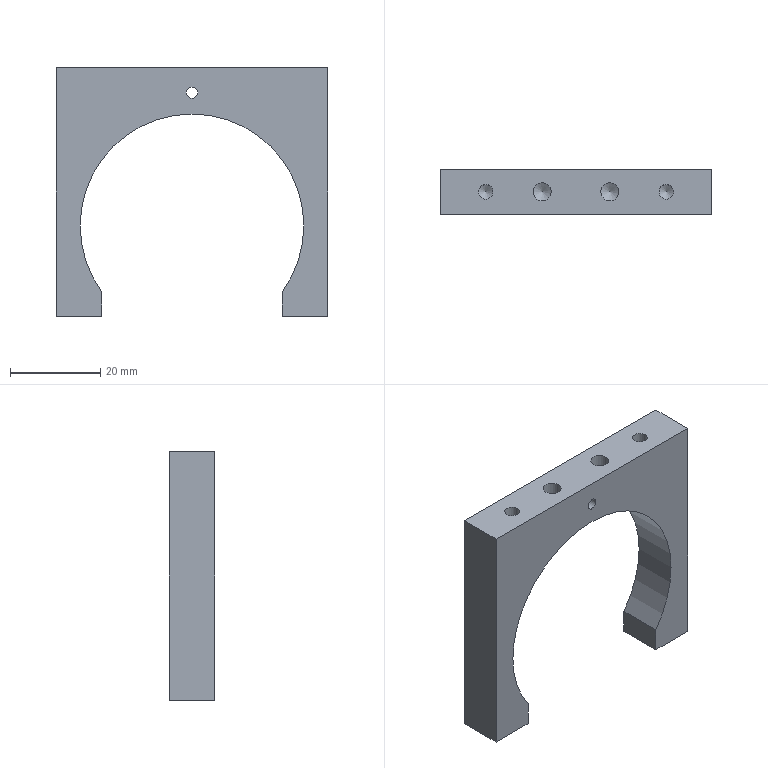Part | STEP file | SynoNew-0304-066 | 1 solid | 23 faces | box 60 x 10 x 55 mm | volume 13958 mm3 | plane 9 | cylinder 8 | cone 6 | commonest cylinder face diameters 2.46 x3 3.24 x2 4 x2 49.5 x1
STEP:
#1=CARTESIAN_POINT('',(0.,0.,-55.));
#2=VERTEX_POINT('',#1);
#3=CARTESIAN_POINT('',(0.,0.,0.));
#4=VERTEX_POINT('',#3);
#5=CARTESIAN_POINT('',(0.,0.,-55.));
#6=DIRECTION('',(0.,0.,1.));
#7=VECTOR('',#6,55.);
#8=LINE('',#5,#7);
#9=EDGE_CURVE('',#2,#4,#8,.T.);
#10=ORIENTED_EDGE('',*,*,#9,.T.);
#11=CARTESIAN_POINT('',(0.,10.,0.));
#12=VERTEX_POINT('',#11);
#13=CARTESIAN_POINT('',(0.,10.,0.));
#14=DIRECTION('',(0.,-1.,0.));
#15=VECTOR('',#14,10.);
#16=LINE('',#13,#15);
#17=EDGE_CURVE('',#12,#4,#16,.T.);
#18=ORIENTED_EDGE('',*,*,#17,.F.);
#19=CARTESIAN_POINT('',(0.,10.,-55.));
#20=VERTEX_POINT('',#19);
#21=CARTESIAN_POINT('',(0.,10.,-55.));
#22=DIRECTION('',(0.,0.,1.));
#23=VECTOR('',#22,55.);
#24=LINE('',#21,#23);
#25=EDGE_CURVE('',#20,#12,#24,.T.);
#26=ORIENTED_EDGE('',*,*,#25,.F.);
#27=CARTESIAN_POINT('',(0.,10.,-55.));
#28=DIRECTION('',(0.,-1.,0.));
#29=VECTOR('',#28,10.);
#30=LINE('',#27,#29);
#31=EDGE_CURVE('',#20,#2,#30,.T.);
#32=ORIENTED_EDGE('',*,*,#31,.T.);
#33=EDGE_LOOP('',(#10,#18,#26,#32));
#34=FACE_OUTER_BOUND('',#33,.T.);
#35=CARTESIAN_POINT('',(0.,10.,0.));
#36=DIRECTION('',(1.,0.,0.));
#37=DIRECTION('',(0.,0.,-1.));
#38=AXIS2_PLACEMENT_3D('',#35,#36,#37);
#39=PLANE('',#38);
#40=ADVANCED_FACE('',(#34),#39,.F.);
#41=CARTESIAN_POINT('',(60.,0.,0.));
#42=VERTEX_POINT('',#41);
#43=CARTESIAN_POINT('',(0.,0.,0.));
#44=DIRECTION('',(1.,0.,0.));
#45=VECTOR('',#44,60.);
#46=LINE('',#43,#45);
#47=EDGE_CURVE('',#4,#42,#46,.T.);
#48=ORIENTED_EDGE('',*,*,#47,.T.);
#49=CARTESIAN_POINT('',(60.,10.,0.));
#50=VERTEX_POINT('',#49);
#51=CARTESIAN_POINT('',(60.,10.,0.));
#52=DIRECTION('',(0.,-1.,0.));
#53=VECTOR('',#52,10.);
#54=LINE('',#51,#53);
#55=EDGE_CURVE('',#50,#42,#54,.T.);
#56=ORIENTED_EDGE('',*,*,#55,.F.);
#57=CARTESIAN_POINT('',(0.,10.,0.));
#58=DIRECTION('',(1.,0.,0.));
#59=VECTOR('',#58,60.);
#60=LINE('',#57,#59);
#61=EDGE_CURVE('',#12,#50,#60,.T.);
#62=ORIENTED_EDGE('',*,*,#61,.F.);
#63=ORIENTED_EDGE('',*,*,#17,.T.);
#64=EDGE_LOOP('',(#48,#56,#62,#63));
#65=FACE_OUTER_BOUND('',#64,.T.);
#66=CARTESIAN_POINT('',(24.5,5.,0.));
#67=VERTEX_POINT('',#66);
#68=CARTESIAN_POINT('',(20.5,5.,0.));
#69=VERTEX_POINT('',#68);
#70=CARTESIAN_POINT('',(22.5,5.,0.));
#71=DIRECTION('',(0.,0.,1.));
#72=DIRECTION('',(1.,0.,0.));
#73=AXIS2_PLACEMENT_3D('',#70,#71,#72);
#74=CIRCLE('',#73,2.);
#75=EDGE_CURVE('',#67,#69,#74,.T.);
#76=ORIENTED_EDGE('',*,*,#75,.F.);
#77=CARTESIAN_POINT('',(22.5,5.,0.));
#78=DIRECTION('',(0.,0.,1.));
#79=DIRECTION('',(1.,0.,0.));
#80=AXIS2_PLACEMENT_3D('',#77,#78,#79);
#81=CIRCLE('',#80,2.);
#82=EDGE_CURVE('',#69,#67,#81,.T.);
#83=ORIENTED_EDGE('',*,*,#82,.F.);
#84=EDGE_LOOP('',(#76,#83));
#85=FACE_BOUND('',#84,.T.);
#86=CARTESIAN_POINT('',(39.5,5.,0.));
#87=VERTEX_POINT('',#86);
#88=CARTESIAN_POINT('',(35.5,5.,0.));
#89=VERTEX_POINT('',#88);
#90=CARTESIAN_POINT('',(37.5,5.,0.));
#91=DIRECTION('',(0.,0.,1.));
#92=DIRECTION('',(1.,0.,0.));
#93=AXIS2_PLACEMENT_3D('',#90,#91,#92);
#94=CIRCLE('',#93,2.);
#95=EDGE_CURVE('',#87,#89,#94,.T.);
#96=ORIENTED_EDGE('',*,*,#95,.F.);
#97=CARTESIAN_POINT('',(37.5,5.,0.));
#98=DIRECTION('',(0.,0.,1.));
#99=DIRECTION('',(1.,0.,0.));
#100=AXIS2_PLACEMENT_3D('',#97,#98,#99);
#101=CIRCLE('',#100,2.);
#102=EDGE_CURVE('',#89,#87,#101,.T.);
#103=ORIENTED_EDGE('',*,*,#102,.F.);
#104=EDGE_LOOP('',(#96,#103));
#105=FACE_BOUND('',#104,.T.);
#106=CARTESIAN_POINT('',(51.62,5.,0.));
#107=VERTEX_POINT('',#106);
#108=CARTESIAN_POINT('',(48.38,5.,0.));
#109=VERTEX_POINT('',#108);
#110=CARTESIAN_POINT('',(50.,5.,0.));
#111=DIRECTION('',(0.,0.,1.));
#112=DIRECTION('',(1.,0.,0.));
#113=AXIS2_PLACEMENT_3D('',#110,#111,#112);
#114=CIRCLE('',#113,1.62);
#115=EDGE_CURVE('',#107,#109,#114,.T.);
#116=ORIENTED_EDGE('',*,*,#115,.F.);
#117=CARTESIAN_POINT('',(50.,5.,0.));
#118=DIRECTION('',(0.,0.,1.));
#119=DIRECTION('',(1.,0.,0.));
#120=AXIS2_PLACEMENT_3D('',#117,#118,#119);
#121=CIRCLE('',#120,1.62);
#122=EDGE_CURVE('',#109,#107,#121,.T.);
#123=ORIENTED_EDGE('',*,*,#122,.F.);
#124=EDGE_LOOP('',(#116,#123));
#125=FACE_BOUND('',#124,.T.);
#126=CARTESIAN_POINT('',(11.62,5.,0.));
#127=VERTEX_POINT('',#126);
#128=CARTESIAN_POINT('',(8.38,5.,0.));
#129=VERTEX_POINT('',#128);
#130=CARTESIAN_POINT('',(10.,5.,0.));
#131=DIRECTION('',(0.,0.,1.));
#132=DIRECTION('',(1.,0.,0.));
#133=AXIS2_PLACEMENT_3D('',#130,#131,#132);
#134=CIRCLE('',#133,1.62);
#135=EDGE_CURVE('',#127,#129,#134,.T.);
#136=ORIENTED_EDGE('',*,*,#135,.F.);
#137=CARTESIAN_POINT('',(10.,5.,0.));
#138=DIRECTION('',(0.,0.,1.));
#139=DIRECTION('',(1.,0.,0.));
#140=AXIS2_PLACEMENT_3D('',#137,#138,#139);
#141=CIRCLE('',#140,1.62);
#142=EDGE_CURVE('',#129,#127,#141,.T.);
#143=ORIENTED_EDGE('',*,*,#142,.F.);
#144=EDGE_LOOP('',(#136,#143));
#145=FACE_BOUND('',#144,.T.);
#146=CARTESIAN_POINT('',(0.,10.,0.));
#147=DIRECTION('',(0.,0.,-1.));
#148=DIRECTION('',(-1.,0.,0.));
#149=AXIS2_PLACEMENT_3D('',#146,#147,#148);
#150=PLANE('',#149);
#151=ADVANCED_FACE('',(#65,#85,#105,#125,#145),#150,.F.);
#152=CARTESIAN_POINT('',(60.,0.,-55.));
#153=VERTEX_POINT('',#152);
#154=CARTESIAN_POINT('',(60.,0.,0.));
#155=DIRECTION('',(0.,0.,-1.));
#156=VECTOR('',#155,55.);
#157=LINE('',#154,#156);
#158=EDGE_CURVE('',#42,#153,#157,.T.);
#159=ORIENTED_EDGE('',*,*,#158,.T.);
#160=CARTESIAN_POINT('',(60.,10.,-55.));
#161=VERTEX_POINT('',#160);
#162=CARTESIAN_POINT('',(60.,10.,-55.));
#163=DIRECTION('',(0.,-1.,0.));
#164=VECTOR('',#163,10.);
#165=LINE('',#162,#164);
#166=EDGE_CURVE('',#161,#153,#165,.T.);
#167=ORIENTED_EDGE('',*,*,#166,.F.);
#168=CARTESIAN_POINT('',(60.,10.,0.));
#169=DIRECTION('',(0.,0.,-1.));
#170=VECTOR('',#169,55.);
#171=LINE('',#168,#170);
#172=EDGE_CURVE('',#50,#161,#171,.T.);
#173=ORIENTED_EDGE('',*,*,#172,.F.);
#174=ORIENTED_EDGE('',*,*,#55,.T.);
#175=EDGE_LOOP('',(#159,#167,#173,#174));
#176=FACE_OUTER_BOUND('',#175,.T.);
#177=CARTESIAN_POINT('',(60.,10.,0.));
#178=DIRECTION('',(-1.,0.,0.));
#179=DIRECTION('',(0.,0.,1.));
#180=AXIS2_PLACEMENT_3D('',#177,#178,#179);
#181=PLANE('',#180);
#182=ADVANCED_FACE('',(#176),#181,.F.);
#183=CARTESIAN_POINT('',(50.,0.,-55.));
#184=VERTEX_POINT('',#183);
#185=CARTESIAN_POINT('',(60.,0.,-55.));
#186=DIRECTION('',(-1.,0.,0.));
#187=VECTOR('',#186,10.);
#188=LINE('',#185,#187);
#189=EDGE_CURVE('',#153,#184,#188,.T.);
#190=ORIENTED_EDGE('',*,*,#189,.T.);
#191=CARTESIAN_POINT('',(50.,10.,-55.));
#192=VERTEX_POINT('',#191);
#193=CARTESIAN_POINT('',(50.,10.,-55.));
#194=DIRECTION('',(0.,-1.,0.));
#195=VECTOR('',#194,10.);
#196=LINE('',#193,#195);
#197=EDGE_CURVE('',#192,#184,#196,.T.);
#198=ORIENTED_EDGE('',*,*,#197,.F.);
#199=CARTESIAN_POINT('',(60.,10.,-55.));
#200=DIRECTION('',(-1.,0.,0.));
#201=VECTOR('',#200,10.);
#202=LINE('',#199,#201);
#203=EDGE_CURVE('',#161,#192,#202,.T.);
#204=ORIENTED_EDGE('',*,*,#203,.F.);
#205=ORIENTED_EDGE('',*,*,#166,.T.);
#206=EDGE_LOOP('',(#190,#198,#204,#205));
#207=FACE_OUTER_BOUND('',#206,.T.);
#208=CARTESIAN_POINT('',(53.77,5.,-55.));
#209=VERTEX_POINT('',#208);
#210=CARTESIAN_POINT('',(56.23,5.,-55.));
#211=VERTEX_POINT('',#210);
#212=CARTESIAN_POINT('',(55.,5.,-55.));
#213=DIRECTION('',(0.,0.,-1.));
#214=DIRECTION('',(-1.,0.,0.));
#215=AXIS2_PLACEMENT_3D('',#212,#213,#214);
#216=CIRCLE('',#215,1.23);
#217=EDGE_CURVE('',#209,#211,#216,.T.);
#218=ORIENTED_EDGE('',*,*,#217,.F.);
#219=CARTESIAN_POINT('',(55.,5.,-55.));
#220=DIRECTION('',(0.,0.,-1.));
#221=DIRECTION('',(-1.,0.,0.));
#222=AXIS2_PLACEMENT_3D('',#219,#220,#221);
#223=CIRCLE('',#222,1.23);
#224=EDGE_CURVE('',#211,#209,#223,.T.);
#225=ORIENTED_EDGE('',*,*,#224,.F.);
#226=EDGE_LOOP('',(#218,#225));
#227=FACE_BOUND('',#226,.T.);
#228=CARTESIAN_POINT('',(50.,10.,-55.));
#229=DIRECTION('',(0.,0.,1.));
#230=DIRECTION('',(1.,0.,0.));
#231=AXIS2_PLACEMENT_3D('',#228,#229,#230);
#232=PLANE('',#231);
#233=ADVANCED_FACE('',(#207,#227),#232,.F.);
#234=CARTESIAN_POINT('',(50.,0.,-49.58));
#235=VERTEX_POINT('',#234);
#236=CARTESIAN_POINT('',(50.,0.,-55.));
#237=DIRECTION('',(0.,0.,1.));
#238=VECTOR('',#237,5.42);
#239=LINE('',#236,#238);
#240=EDGE_CURVE('',#184,#235,#239,.T.);
#241=ORIENTED_EDGE('',*,*,#240,.T.);
#242=CARTESIAN_POINT('',(50.,10.,-49.58));
#243=VERTEX_POINT('',#242);
#244=CARTESIAN_POINT('',(50.,10.,-49.58));
#245=DIRECTION('',(0.,-1.,0.));
#246=VECTOR('',#245,10.);
#247=LINE('',#244,#246);
#248=EDGE_CURVE('',#243,#235,#247,.T.);
#249=ORIENTED_EDGE('',*,*,#248,.F.);
#250=CARTESIAN_POINT('',(50.,10.,-55.));
#251=DIRECTION('',(0.,0.,1.));
#252=VECTOR('',#251,5.42);
#253=LINE('',#250,#252);
#254=EDGE_CURVE('',#192,#243,#253,.T.);
#255=ORIENTED_EDGE('',*,*,#254,.F.);
#256=ORIENTED_EDGE('',*,*,#197,.T.);
#257=EDGE_LOOP('',(#241,#249,#255,#256));
#258=FACE_OUTER_BOUND('',#257,.T.);
#259=CARTESIAN_POINT('',(50.,10.,-55.));
#260=DIRECTION('',(1.,0.,0.));
#261=DIRECTION('',(0.,0.,-1.));
#262=AXIS2_PLACEMENT_3D('',#259,#260,#261);
#263=PLANE('',#262);
#264=ADVANCED_FACE('',(#258),#263,.F.);
#265=CARTESIAN_POINT('',(10.,0.,-49.58));
#266=VERTEX_POINT('',#265);
#267=CARTESIAN_POINT('',(30.,0.,-35.));
#268=DIRECTION('',(0.,-1.,0.));
#269=DIRECTION('',(0.,0.,1.));
#270=AXIS2_PLACEMENT_3D('',#267,#268,#269);
#271=CIRCLE('',#270,24.75);
#272=EDGE_CURVE('',#235,#266,#271,.T.);
#273=ORIENTED_EDGE('',*,*,#272,.T.);
#274=CARTESIAN_POINT('',(10.,10.,-49.58));
#275=VERTEX_POINT('',#274);
#276=CARTESIAN_POINT('',(10.,10.,-49.58));
#277=DIRECTION('',(0.,-1.,0.));
#278=VECTOR('',#277,10.);
#279=LINE('',#276,#278);
#280=EDGE_CURVE('',#275,#266,#279,.T.);
#281=ORIENTED_EDGE('',*,*,#280,.F.);
#282=CARTESIAN_POINT('',(30.,10.,-35.));
#283=DIRECTION('',(0.,-1.,0.));
#284=DIRECTION('',(0.,0.,1.));
#285=AXIS2_PLACEMENT_3D('',#282,#283,#284);
#286=CIRCLE('',#285,24.75);
#287=EDGE_CURVE('',#243,#275,#286,.T.);
#288=ORIENTED_EDGE('',*,*,#287,.F.);
#289=ORIENTED_EDGE('',*,*,#248,.T.);
#290=EDGE_LOOP('',(#273,#281,#288,#289));
#291=FACE_OUTER_BOUND('',#290,.T.);
#292=CARTESIAN_POINT('',(30.,10.,-35.));
#293=DIRECTION('',(0.,-1.,0.));
#294=DIRECTION('',(0.,0.,1.));
#295=AXIS2_PLACEMENT_3D('',#292,#293,#294);
#296=CYLINDRICAL_SURFACE('',#295,24.75);
#297=ADVANCED_FACE('',(#291),#296,.F.);
#298=CARTESIAN_POINT('',(10.,0.,-55.));
#299=VERTEX_POINT('',#298);
#300=CARTESIAN_POINT('',(10.,0.,-49.58));
#301=DIRECTION('',(0.,0.,-1.));
#302=VECTOR('',#301,5.42);
#303=LINE('',#300,#302);
#304=EDGE_CURVE('',#266,#299,#303,.T.);
#305=ORIENTED_EDGE('',*,*,#304,.T.);
#306=CARTESIAN_POINT('',(10.,10.,-55.));
#307=VERTEX_POINT('',#306);
#308=CARTESIAN_POINT('',(10.,10.,-55.));
#309=DIRECTION('',(0.,-1.,0.));
#310=VECTOR('',#309,10.);
#311=LINE('',#308,#310);
#312=EDGE_CURVE('',#307,#299,#311,.T.);
#313=ORIENTED_EDGE('',*,*,#312,.F.);
#314=CARTESIAN_POINT('',(10.,10.,-49.58));
#315=DIRECTION('',(0.,0.,-1.));
#316=VECTOR('',#315,5.42);
#317=LINE('',#314,#316);
#318=EDGE_CURVE('',#275,#307,#317,.T.);
#319=ORIENTED_EDGE('',*,*,#318,.F.);
#320=ORIENTED_EDGE('',*,*,#280,.T.);
#321=EDGE_LOOP('',(#305,#313,#319,#320));
#322=FACE_OUTER_BOUND('',#321,.T.);
#323=CARTESIAN_POINT('',(10.,10.,-55.));
#324=DIRECTION('',(-1.,0.,0.));
#325=DIRECTION('',(0.,0.,1.));
#326=AXIS2_PLACEMENT_3D('',#323,#324,#325);
#327=PLANE('',#326);
#328=ADVANCED_FACE('',(#322),#327,.F.);
#329=CARTESIAN_POINT('',(10.,0.,-55.));
#330=DIRECTION('',(-1.,0.,0.));
#331=VECTOR('',#330,10.);
#332=LINE('',#329,#331);
#333=EDGE_CURVE('',#299,#2,#332,.T.);
#334=ORIENTED_EDGE('',*,*,#333,.T.);
#335=ORIENTED_EDGE('',*,*,#31,.F.);
#336=CARTESIAN_POINT('',(10.,10.,-55.));
#337=DIRECTION('',(-1.,0.,0.));
#338=VECTOR('',#337,10.);
#339=LINE('',#336,#338);
#340=EDGE_CURVE('',#307,#20,#339,.T.);
#341=ORIENTED_EDGE('',*,*,#340,.F.);
#342=ORIENTED_EDGE('',*,*,#312,.T.);
#343=EDGE_LOOP('',(#334,#335,#341,#342));
#344=FACE_OUTER_BOUND('',#343,.T.);
#345=CARTESIAN_POINT('',(3.77,5.,-55.));
#346=VERTEX_POINT('',#345);
#347=CARTESIAN_POINT('',(6.23,5.,-55.));
#348=VERTEX_POINT('',#347);
#349=CARTESIAN_POINT('',(5.,5.,-55.));
#350=DIRECTION('',(0.,0.,-1.));
#351=DIRECTION('',(-1.,0.,0.));
#352=AXIS2_PLACEMENT_3D('',#349,#350,#351);
#353=CIRCLE('',#352,1.23);
#354=EDGE_CURVE('',#346,#348,#353,.T.);
#355=ORIENTED_EDGE('',*,*,#354,.F.);
#356=CARTESIAN_POINT('',(5.,5.,-55.));
#357=DIRECTION('',(0.,0.,-1.));
#358=DIRECTION('',(-1.,0.,0.));
#359=AXIS2_PLACEMENT_3D('',#356,#357,#358);
#360=CIRCLE('',#359,1.23);
#361=EDGE_CURVE('',#348,#346,#360,.T.);
#362=ORIENTED_EDGE('',*,*,#361,.F.);
#363=EDGE_LOOP('',(#355,#362));
#364=FACE_BOUND('',#363,.T.);
#365=CARTESIAN_POINT('',(0.,10.,-55.));
#366=DIRECTION('',(0.,0.,1.));
#367=DIRECTION('',(1.,0.,0.));
#368=AXIS2_PLACEMENT_3D('',#365,#366,#367);
#369=PLANE('',#368);
#370=ADVANCED_FACE('',(#344,#364),#369,.F.);
#371=ORIENTED_EDGE('',*,*,#25,.T.);
#372=ORIENTED_EDGE('',*,*,#61,.T.);
#373=ORIENTED_EDGE('',*,*,#172,.T.);
#374=ORIENTED_EDGE('',*,*,#203,.T.);
#375=ORIENTED_EDGE('',*,*,#254,.T.);
#376=ORIENTED_EDGE('',*,*,#287,.T.);
#377=ORIENTED_EDGE('',*,*,#318,.T.);
#378=ORIENTED_EDGE('',*,*,#340,.T.);
#379=EDGE_LOOP('',(#371,#372,#373,#374,#375,#376,#377,#378));
#380=FACE_OUTER_BOUND('',#379,.T.);
#381=CARTESIAN_POINT('',(30.,10.,-4.27));
#382=VERTEX_POINT('',#381);
#383=CARTESIAN_POINT('',(30.,10.,-6.73));
#384=VERTEX_POINT('',#383);
#385=CARTESIAN_POINT('',(30.,10.,-5.5));
#386=DIRECTION('',(0.,1.,0.));
#387=DIRECTION('',(0.,0.,1.));
#388=AXIS2_PLACEMENT_3D('',#385,#386,#387);
#389=CIRCLE('',#388,1.23);
#390=EDGE_CURVE('',#382,#384,#389,.T.);
#391=ORIENTED_EDGE('',*,*,#390,.F.);
#392=CARTESIAN_POINT('',(30.,10.,-5.5));
#393=DIRECTION('',(0.,1.,0.));
#394=DIRECTION('',(0.,0.,1.));
#395=AXIS2_PLACEMENT_3D('',#392,#393,#394);
#396=CIRCLE('',#395,1.23);
#397=EDGE_CURVE('',#384,#382,#396,.T.);
#398=ORIENTED_EDGE('',*,*,#397,.F.);
#399=EDGE_LOOP('',(#391,#398));
#400=FACE_BOUND('',#399,.T.);
#401=CARTESIAN_POINT('',(30.,10.,-35.));
#402=DIRECTION('',(0.,1.,0.));
#403=DIRECTION('',(0.,0.,1.));
#404=AXIS2_PLACEMENT_3D('',#401,#402,#403);
#405=PLANE('',#404);
#406=ADVANCED_FACE('',(#380,#400),#405,.T.);
#407=ORIENTED_EDGE('',*,*,#9,.F.);
#408=ORIENTED_EDGE('',*,*,#333,.F.);
#409=ORIENTED_EDGE('',*,*,#304,.F.);
#410=ORIENTED_EDGE('',*,*,#272,.F.);
#411=ORIENTED_EDGE('',*,*,#240,.F.);
#412=ORIENTED_EDGE('',*,*,#189,.F.);
#413=ORIENTED_EDGE('',*,*,#158,.F.);
#414=ORIENTED_EDGE('',*,*,#47,.F.);
#415=EDGE_LOOP('',(#407,#408,#409,#410,#411,#412,#413,#414));
#416=FACE_OUTER_BOUND('',#415,.T.);
#417=CARTESIAN_POINT('',(30.,0.,-4.27));
#418=VERTEX_POINT('',#417);
#419=CARTESIAN_POINT('',(30.,0.,-6.73));
#420=VERTEX_POINT('',#419);
#421=CARTESIAN_POINT('',(30.,0.,-5.5));
#422=DIRECTION('',(0.,1.,0.));
#423=DIRECTION('',(0.,0.,1.));
#424=AXIS2_PLACEMENT_3D('',#421,#422,#423);
#425=CIRCLE('',#424,1.23);
#426=EDGE_CURVE('',#418,#420,#425,.T.);
#427=ORIENTED_EDGE('',*,*,#426,.T.);
#428=CARTESIAN_POINT('',(30.,0.,-5.5));
#429=DIRECTION('',(0.,1.,0.));
#430=DIRECTION('',(0.,0.,1.));
#431=AXIS2_PLACEMENT_3D('',#428,#429,#430);
#432=CIRCLE('',#431,1.23);
#433=EDGE_CURVE('',#420,#418,#432,.T.);
#434=ORIENTED_EDGE('',*,*,#433,.T.);
#435=EDGE_LOOP('',(#427,#434));
#436=FACE_BOUND('',#435,.T.);
#437=CARTESIAN_POINT('',(30.,0.,-35.));
#438=DIRECTION('',(0.,1.,0.));
#439=DIRECTION('',(0.,0.,1.));
#440=AXIS2_PLACEMENT_3D('',#437,#438,#439);
#441=PLANE('',#440);
#442=ADVANCED_FACE('',(#416,#436),#441,.F.);
#443=CARTESIAN_POINT('',(10.,5.,-12.473));
#444=VERTEX_POINT('',#443);
#445=CARTESIAN_POINT('',(8.38,5.,-11.5));
#446=VERTEX_POINT('',#445);
#447=CARTESIAN_POINT('',(8.38,5.,-11.5));
#448=DIRECTION('',(-0.8572,0.,0.515));
#449=VECTOR('',#448,1.62);
#450=LINE('',#447,#449);
#451=EDGE_CURVE('',#444,#446,#450,.T.);
#452=ORIENTED_EDGE('',*,*,#451,.T.);
#453=CARTESIAN_POINT('',(11.62,5.,-11.5));
#454=VERTEX_POINT('',#453);
#455=CARTESIAN_POINT('',(10.,5.,-11.5));
#456=DIRECTION('',(0.,0.,1.));
#457=DIRECTION('',(1.,0.,0.));
#458=AXIS2_PLACEMENT_3D('',#455,#456,#457);
#459=CIRCLE('',#458,1.62);
#460=EDGE_CURVE('',#446,#454,#459,.T.);
#461=ORIENTED_EDGE('',*,*,#460,.T.);
#462=CARTESIAN_POINT('',(10.,5.,-11.5));
#463=DIRECTION('',(0.,0.,1.));
#464=DIRECTION('',(1.,0.,0.));
#465=AXIS2_PLACEMENT_3D('',#462,#463,#464);
#466=CIRCLE('',#465,1.62);
#467=EDGE_CURVE('',#454,#446,#466,.T.);
#468=ORIENTED_EDGE('',*,*,#467,.T.);
#469=ORIENTED_EDGE('',*,*,#451,.F.);
#470=EDGE_LOOP('',(#452,#461,#468,#469));
#471=FACE_OUTER_BOUND('',#470,.T.);
#472=CARTESIAN_POINT('',(10.,5.,-11.5));
#473=DIRECTION('',(0.,0.,1.));
#474=DIRECTION('',(1.,0.,0.));
#475=AXIS2_PLACEMENT_3D('',#472,#473,#474);
#476=CONICAL_SURFACE('',#475,1.62,1.03);
#477=ADVANCED_FACE('',(#471),#476,.F.);
#478=ORIENTED_EDGE('',*,*,#467,.F.);
#479=ORIENTED_EDGE('',*,*,#460,.F.);
#480=CARTESIAN_POINT('',(8.38,5.,0.));
#481=DIRECTION('',(0.,0.,1.));
#482=VECTOR('',#481,1.62);
#483=LINE('',#480,#482);
#484=EDGE_CURVE('',#446,#129,#483,.T.);
#485=ORIENTED_EDGE('',*,*,#484,.T.);
#486=ORIENTED_EDGE('',*,*,#142,.T.);
#487=ORIENTED_EDGE('',*,*,#135,.T.);
#488=ORIENTED_EDGE('',*,*,#484,.F.);
#489=EDGE_LOOP('',(#478,#479,#485,#486,#487,#488));
#490=FACE_OUTER_BOUND('',#489,.T.);
#491=CARTESIAN_POINT('',(10.,5.,0.));
#492=DIRECTION('',(0.,0.,1.));
#493=DIRECTION('',(1.,0.,0.));
#494=AXIS2_PLACEMENT_3D('',#491,#492,#493);
#495=CYLINDRICAL_SURFACE('',#494,1.62);
#496=ADVANCED_FACE('',(#490),#495,.F.);
#497=CARTESIAN_POINT('',(50.,5.,-12.473));
#498=VERTEX_POINT('',#497);
#499=CARTESIAN_POINT('',(48.38,5.,-11.5));
#500=VERTEX_POINT('',#499);
#501=CARTESIAN_POINT('',(48.38,5.,-11.5));
#502=DIRECTION('',(-0.8572,0.,0.515));
#503=VECTOR('',#502,1.62);
#504=LINE('',#501,#503);
#505=EDGE_CURVE('',#498,#500,#504,.T.);
#506=ORIENTED_EDGE('',*,*,#505,.T.);
#507=CARTESIAN_POINT('',(51.62,5.,-11.5));
#508=VERTEX_POINT('',#507);
#509=CARTESIAN_POINT('',(50.,5.,-11.5));
#510=DIRECTION('',(0.,0.,1.));
#511=DIRECTION('',(1.,0.,0.));
#512=AXIS2_PLACEMENT_3D('',#509,#510,#511);
#513=CIRCLE('',#512,1.62);
#514=EDGE_CURVE('',#500,#508,#513,.T.);
#515=ORIENTED_EDGE('',*,*,#514,.T.);
#516=CARTESIAN_POINT('',(50.,5.,-11.5));
#517=DIRECTION('',(0.,0.,1.));
#518=DIRECTION('',(1.,0.,0.));
#519=AXIS2_PLACEMENT_3D('',#516,#517,#518);
#520=CIRCLE('',#519,1.62);
#521=EDGE_CURVE('',#508,#500,#520,.T.);
#522=ORIENTED_EDGE('',*,*,#521,.T.);
#523=ORIENTED_EDGE('',*,*,#505,.F.);
#524=EDGE_LOOP('',(#506,#515,#522,#523));
#525=FACE_OUTER_BOUND('',#524,.T.);
#526=CARTESIAN_POINT('',(50.,5.,-11.5));
#527=DIRECTION('',(0.,0.,1.));
#528=DIRECTION('',(1.,0.,0.));
#529=AXIS2_PLACEMENT_3D('',#526,#527,#528);
#530=CONICAL_SURFACE('',#529,1.62,1.03);
#531=ADVANCED_FACE('',(#525),#530,.F.);
#532=ORIENTED_EDGE('',*,*,#521,.F.);
#533=ORIENTED_EDGE('',*,*,#514,.F.);
#534=CARTESIAN_POINT('',(48.38,5.,0.));
#535=DIRECTION('',(0.,0.,1.));
#536=VECTOR('',#535,1.62);
#537=LINE('',#534,#536);
#538=EDGE_CURVE('',#500,#109,#537,.T.);
#539=ORIENTED_EDGE('',*,*,#538,.T.);
#540=ORIENTED_EDGE('',*,*,#122,.T.);
#541=ORIENTED_EDGE('',*,*,#115,.T.);
#542=ORIENTED_EDGE('',*,*,#538,.F.);
#543=EDGE_LOOP('',(#532,#533,#539,#540,#541,#542));
#544=FACE_OUTER_BOUND('',#543,.T.);
#545=CARTESIAN_POINT('',(50.,5.,0.));
#546=DIRECTION('',(0.,0.,1.));
#547=DIRECTION('',(1.,0.,0.));
#548=AXIS2_PLACEMENT_3D('',#545,#546,#547);
#549=CYLINDRICAL_SURFACE('',#548,1.62);
#550=ADVANCED_FACE('',(#544),#549,.F.);
#551=CARTESIAN_POINT('',(37.5,5.,-7.202));
#552=VERTEX_POINT('',#551);
#553=CARTESIAN_POINT('',(35.5,5.,-6.));
#554=VERTEX_POINT('',#553);
#555=CARTESIAN_POINT('',(35.5,5.,-6.));
#556=DIRECTION('',(-0.8572,0.,0.515));
#557=VECTOR('',#556,2.);
#558=LINE('',#555,#557);
#559=EDGE_CURVE('',#552,#554,#558,.T.);
#560=ORIENTED_EDGE('',*,*,#559,.T.);
#561=CARTESIAN_POINT('',(39.5,5.,-6.));
#562=VERTEX_POINT('',#561);
#563=CARTESIAN_POINT('',(37.5,5.,-6.));
#564=DIRECTION('',(0.,0.,1.));
#565=DIRECTION('',(1.,0.,0.));
#566=AXIS2_PLACEMENT_3D('',#563,#564,#565);
#567=CIRCLE('',#566,2.);
#568=EDGE_CURVE('',#554,#562,#567,.T.);
#569=ORIENTED_EDGE('',*,*,#568,.T.);
#570=CARTESIAN_POINT('',(37.5,5.,-6.));
#571=DIRECTION('',(0.,0.,1.));
#572=DIRECTION('',(1.,0.,0.));
#573=AXIS2_PLACEMENT_3D('',#570,#571,#572);
#574=CIRCLE('',#573,2.);
#575=EDGE_CURVE('',#562,#554,#574,.T.);
#576=ORIENTED_EDGE('',*,*,#575,.T.);
#577=ORIENTED_EDGE('',*,*,#559,.F.);
#578=EDGE_LOOP('',(#560,#569,#576,#577));
#579=FACE_OUTER_BOUND('',#578,.T.);
#580=CARTESIAN_POINT('',(37.5,5.,-6.));
#581=DIRECTION('',(0.,0.,1.));
#582=DIRECTION('',(1.,0.,0.));
#583=AXIS2_PLACEMENT_3D('',#580,#581,#582);
#584=CONICAL_SURFACE('',#583,2.,1.03);
#585=ADVANCED_FACE('',(#579),#584,.F.);
#586=ORIENTED_EDGE('',*,*,#575,.F.);
#587=ORIENTED_EDGE('',*,*,#568,.F.);
#588=CARTESIAN_POINT('',(35.5,5.,0.));
#589=DIRECTION('',(0.,0.,1.));
#590=VECTOR('',#589,2.);
#591=LINE('',#588,#590);
#592=EDGE_CURVE('',#554,#89,#591,.T.);
#593=ORIENTED_EDGE('',*,*,#592,.T.);
#594=ORIENTED_EDGE('',*,*,#102,.T.);
#595=ORIENTED_EDGE('',*,*,#95,.T.);
#596=ORIENTED_EDGE('',*,*,#592,.F.);
#597=EDGE_LOOP('',(#586,#587,#593,#594,#595,#596));
#598=FACE_OUTER_BOUND('',#597,.T.);
#599=CARTESIAN_POINT('',(37.5,5.,0.));
#600=DIRECTION('',(0.,0.,1.));
#601=DIRECTION('',(1.,0.,0.));
#602=AXIS2_PLACEMENT_3D('',#599,#600,#601);
#603=CYLINDRICAL_SURFACE('',#602,2.);
#604=ADVANCED_FACE('',(#598),#603,.F.);
#605=CARTESIAN_POINT('',(22.5,5.,-7.202));
#606=VERTEX_POINT('',#605);
#607=CARTESIAN_POINT('',(20.5,5.,-6.));
#608=VERTEX_POINT('',#607);
#609=CARTESIAN_POINT('',(20.5,5.,-6.));
#610=DIRECTION('',(-0.8572,0.,0.515));
#611=VECTOR('',#610,2.);
#612=LINE('',#609,#611);
#613=EDGE_CURVE('',#606,#608,#612,.T.);
#614=ORIENTED_EDGE('',*,*,#613,.T.);
#615=CARTESIAN_POINT('',(24.5,5.,-6.));
#616=VERTEX_POINT('',#615);
#617=CARTESIAN_POINT('',(22.5,5.,-6.));
#618=DIRECTION('',(0.,0.,1.));
#619=DIRECTION('',(1.,0.,0.));
#620=AXIS2_PLACEMENT_3D('',#617,#618,#619);
#621=CIRCLE('',#620,2.);
#622=EDGE_CURVE('',#608,#616,#621,.T.);
#623=ORIENTED_EDGE('',*,*,#622,.T.);
#624=CARTESIAN_POINT('',(22.5,5.,-6.));
#625=DIRECTION('',(0.,0.,1.));
#626=DIRECTION('',(1.,0.,0.));
#627=AXIS2_PLACEMENT_3D('',#624,#625,#626);
#628=CIRCLE('',#627,2.);
#629=EDGE_CURVE('',#616,#608,#628,.T.);
#630=ORIENTED_EDGE('',*,*,#629,.T.);
#631=ORIENTED_EDGE('',*,*,#613,.F.);
#632=EDGE_LOOP('',(#614,#623,#630,#631));
#633=FACE_OUTER_BOUND('',#632,.T.);
#634=CARTESIAN_POINT('',(22.5,5.,-6.));
#635=DIRECTION('',(0.,0.,1.));
#636=DIRECTION('',(1.,0.,0.));
#637=AXIS2_PLACEMENT_3D('',#634,#635,#636);
#638=CONICAL_SURFACE('',#637,2.,1.03);
#639=ADVANCED_FACE('',(#633),#638,.F.);
#640=ORIENTED_EDGE('',*,*,#629,.F.);
#641=ORIENTED_EDGE('',*,*,#622,.F.);
#642=CARTESIAN_POINT('',(20.5,5.,0.));
#643=DIRECTION('',(0.,0.,1.));
#644=VECTOR('',#643,2.);
#645=LINE('',#642,#644);
#646=EDGE_CURVE('',#608,#69,#645,.T.);
#647=ORIENTED_EDGE('',*,*,#646,.T.);
#648=ORIENTED_EDGE('',*,*,#82,.T.);
#649=ORIENTED_EDGE('',*,*,#75,.T.);
#650=ORIENTED_EDGE('',*,*,#646,.F.);
#651=EDGE_LOOP('',(#640,#641,#647,#648,#649,#650));
#652=FACE_OUTER_BOUND('',#651,.T.);
#653=CARTESIAN_POINT('',(22.5,5.,0.));
#654=DIRECTION('',(0.,0.,1.));
#655=DIRECTION('',(1.,0.,0.));
#656=AXIS2_PLACEMENT_3D('',#653,#654,#655);
#657=CYLINDRICAL_SURFACE('',#656,2.);
#658=ADVANCED_FACE('',(#652),#657,.F.);
#659=CARTESIAN_POINT('',(55.,5.,-46.761));
#660=VERTEX_POINT('',#659);
#661=CARTESIAN_POINT('',(56.23,5.,-47.5));
#662=VERTEX_POINT('',#661);
#663=CARTESIAN_POINT('',(56.23,5.,-47.5));
#664=DIRECTION('',(0.8572,0.,-0.515));
#665=VECTOR('',#664,1.23);
#666=LINE('',#663,#665);
#667=EDGE_CURVE('',#660,#662,#666,.T.);
#668=ORIENTED_EDGE('',*,*,#667,.T.);
#669=CARTESIAN_POINT('',(53.77,5.,-47.5));
#670=VERTEX_POINT('',#669);
#671=CARTESIAN_POINT('',(55.,5.,-47.5));
#672=DIRECTION('',(0.,0.,-1.));
#673=DIRECTION('',(-1.,0.,0.));
#674=AXIS2_PLACEMENT_3D('',#671,#672,#673);
#675=CIRCLE('',#674,1.23);
#676=EDGE_CURVE('',#662,#670,#675,.T.);
#677=ORIENTED_EDGE('',*,*,#676,.T.);
#678=CARTESIAN_POINT('',(55.,5.,-47.5));
#679=DIRECTION('',(0.,0.,-1.));
#680=DIRECTION('',(-1.,0.,0.));
#681=AXIS2_PLACEMENT_3D('',#678,#679,#680);
#682=CIRCLE('',#681,1.23);
#683=EDGE_CURVE('',#670,#662,#682,.T.);
#684=ORIENTED_EDGE('',*,*,#683,.T.);
#685=ORIENTED_EDGE('',*,*,#667,.F.);
#686=EDGE_LOOP('',(#668,#677,#684,#685));
#687=FACE_OUTER_BOUND('',#686,.T.);
#688=CARTESIAN_POINT('',(55.,5.,-47.5));
#689=DIRECTION('',(0.,0.,-1.));
#690=DIRECTION('',(-1.,0.,0.));
#691=AXIS2_PLACEMENT_3D('',#688,#689,#690);
#692=CONICAL_SURFACE('',#691,1.23,1.03);
#693=ADVANCED_FACE('',(#687),#692,.F.);
#694=ORIENTED_EDGE('',*,*,#683,.F.);
#695=ORIENTED_EDGE('',*,*,#676,.F.);
#696=CARTESIAN_POINT('',(56.23,5.,-55.));
#697=DIRECTION('',(0.,0.,-1.));
#698=VECTOR('',#697,1.23);
#699=LINE('',#696,#698);
#700=EDGE_CURVE('',#662,#211,#699,.T.);
#701=ORIENTED_EDGE('',*,*,#700,.T.);
#702=ORIENTED_EDGE('',*,*,#224,.T.);
#703=ORIENTED_EDGE('',*,*,#217,.T.);
#704=ORIENTED_EDGE('',*,*,#700,.F.);
#705=EDGE_LOOP('',(#694,#695,#701,#702,#703,#704));
#706=FACE_OUTER_BOUND('',#705,.T.);
#707=CARTESIAN_POINT('',(55.,5.,-55.));
#708=DIRECTION('',(0.,0.,-1.));
#709=DIRECTION('',(-1.,0.,0.));
#710=AXIS2_PLACEMENT_3D('',#707,#708,#709);
#711=CYLINDRICAL_SURFACE('',#710,1.23);
#712=ADVANCED_FACE('',(#706),#711,.F.);
#713=CARTESIAN_POINT('',(5.,5.,-46.761));
#714=VERTEX_POINT('',#713);
#715=CARTESIAN_POINT('',(6.23,5.,-47.5));
#716=VERTEX_POINT('',#715);
#717=CARTESIAN_POINT('',(6.23,5.,-47.5));
#718=DIRECTION('',(0.8572,0.,-0.515));
#719=VECTOR('',#718,1.23);
#720=LINE('',#717,#719);
#721=EDGE_CURVE('',#714,#716,#720,.T.);
#722=ORIENTED_EDGE('',*,*,#721,.T.);
#723=CARTESIAN_POINT('',(3.77,5.,-47.5));
#724=VERTEX_POINT('',#723);
#725=CARTESIAN_POINT('',(5.,5.,-47.5));
#726=DIRECTION('',(0.,0.,-1.));
#727=DIRECTION('',(-1.,0.,0.));
#728=AXIS2_PLACEMENT_3D('',#725,#726,#727);
#729=CIRCLE('',#728,1.23);
#730=EDGE_CURVE('',#716,#724,#729,.T.);
#731=ORIENTED_EDGE('',*,*,#730,.T.);
#732=CARTESIAN_POINT('',(5.,5.,-47.5));
#733=DIRECTION('',(0.,0.,-1.));
#734=DIRECTION('',(-1.,0.,0.));
#735=AXIS2_PLACEMENT_3D('',#732,#733,#734);
#736=CIRCLE('',#735,1.23);
#737=EDGE_CURVE('',#724,#716,#736,.T.);
#738=ORIENTED_EDGE('',*,*,#737,.T.);
#739=ORIENTED_EDGE('',*,*,#721,.F.);
#740=EDGE_LOOP('',(#722,#731,#738,#739));
#741=FACE_OUTER_BOUND('',#740,.T.);
#742=CARTESIAN_POINT('',(5.,5.,-47.5));
#743=DIRECTION('',(0.,0.,-1.));
#744=DIRECTION('',(-1.,0.,0.));
#745=AXIS2_PLACEMENT_3D('',#742,#743,#744);
#746=CONICAL_SURFACE('',#745,1.23,1.03);
#747=ADVANCED_FACE('',(#741),#746,.F.);
#748=ORIENTED_EDGE('',*,*,#737,.F.);
#749=ORIENTED_EDGE('',*,*,#730,.F.);
#750=CARTESIAN_POINT('',(6.23,5.,-55.));
#751=DIRECTION('',(0.,0.,-1.));
#752=VECTOR('',#751,1.23);
#753=LINE('',#750,#752);
#754=EDGE_CURVE('',#716,#348,#753,.T.);
#755=ORIENTED_EDGE('',*,*,#754,.T.);
#756=ORIENTED_EDGE('',*,*,#361,.T.);
#757=ORIENTED_EDGE('',*,*,#354,.T.);
#758=ORIENTED_EDGE('',*,*,#754,.F.);
#759=EDGE_LOOP('',(#748,#749,#755,#756,#757,#758));
#760=FACE_OUTER_BOUND('',#759,.T.);
#761=CARTESIAN_POINT('',(5.,5.,-55.));
#762=DIRECTION('',(0.,0.,-1.));
#763=DIRECTION('',(-1.,0.,0.));
#764=AXIS2_PLACEMENT_3D('',#761,#762,#763);
#765=CYLINDRICAL_SURFACE('',#764,1.23);
#766=ADVANCED_FACE('',(#760),#765,.F.);
#767=ORIENTED_EDGE('',*,*,#426,.F.);
#768=ORIENTED_EDGE('',*,*,#433,.F.);
#769=CARTESIAN_POINT('',(30.,10.,-6.73));
#770=DIRECTION('',(0.,1.,0.));
#771=VECTOR('',#770,1.23);
#772=LINE('',#769,#771);
#773=EDGE_CURVE('',#420,#384,#772,.T.);
#774=ORIENTED_EDGE('',*,*,#773,.T.);
#775=ORIENTED_EDGE('',*,*,#397,.T.);
#776=ORIENTED_EDGE('',*,*,#390,.T.);
#777=ORIENTED_EDGE('',*,*,#773,.F.);
#778=EDGE_LOOP('',(#767,#768,#774,#775,#776,#777));
#779=FACE_OUTER_BOUND('',#778,.T.);
#780=CARTESIAN_POINT('',(30.,10.,-5.5));
#781=DIRECTION('',(0.,1.,0.));
#782=DIRECTION('',(0.,0.,1.));
#783=AXIS2_PLACEMENT_3D('',#780,#781,#782);
#784=CYLINDRICAL_SURFACE('',#783,1.23);
#785=ADVANCED_FACE('',(#779),#784,.F.);
#786=CLOSED_SHELL('',(#40,#151,#182,#233,#264,#297,#328,#370,#406,#442,#477,#496,#531,#550,#585,#604,#639,#658,#693,#712,#747,#766,#785));
#787=MANIFOLD_SOLID_BREP('',#786);
#788=(LENGTH_UNIT()NAMED_UNIT(*)SI_UNIT(.MILLI.,.METRE.));
#789=UNCERTAINTY_MEASURE_WITH_UNIT(LENGTH_MEASURE(0.01),#788,'','');
#790=(NAMED_UNIT(*)PLANE_ANGLE_UNIT()SI_UNIT($,.RADIAN.));
#791=(NAMED_UNIT(*)SI_UNIT($,.STERADIAN.)SOLID_ANGLE_UNIT());
#792=(GEOMETRIC_REPRESENTATION_CONTEXT(3)GLOBAL_UNCERTAINTY_ASSIGNED_CONTEXT((#789))GLOBAL_UNIT_ASSIGNED_CONTEXT((#788,#790,#791))REPRESENTATION_CONTEXT('',''));
#793=ADVANCED_BREP_SHAPE_REPRESENTATION('',(#787),#792);